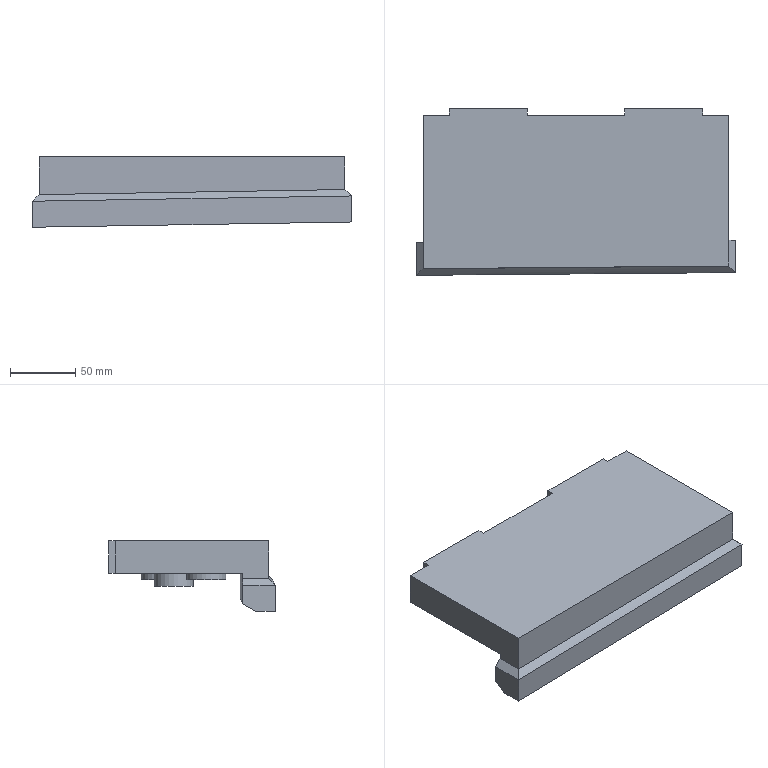Part | NX | features solid 2 | 1 solid | 33 faces | box 245 x 127.987 x 54.158 mm | volume 879012 mm3 | plane 22 | spline 6 | cylinder 5 | commonest cylinder face diameters 30 x5